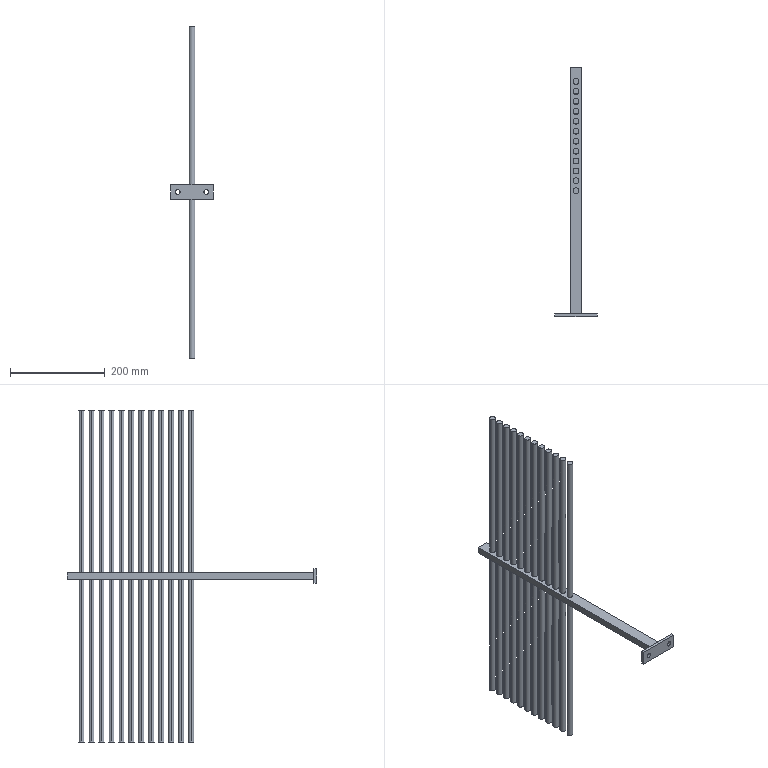Part | SolidWorks | features ICE 4, Extrusion 1, HoleWzd 1, LPattern 1 | 1 solid | 87 faces | box 90 x 526 x 700 mm | volume 1128275 mm3 | cylinder 52 | plane 35 | commonest cylinder face diameters 12 x48 10 x4